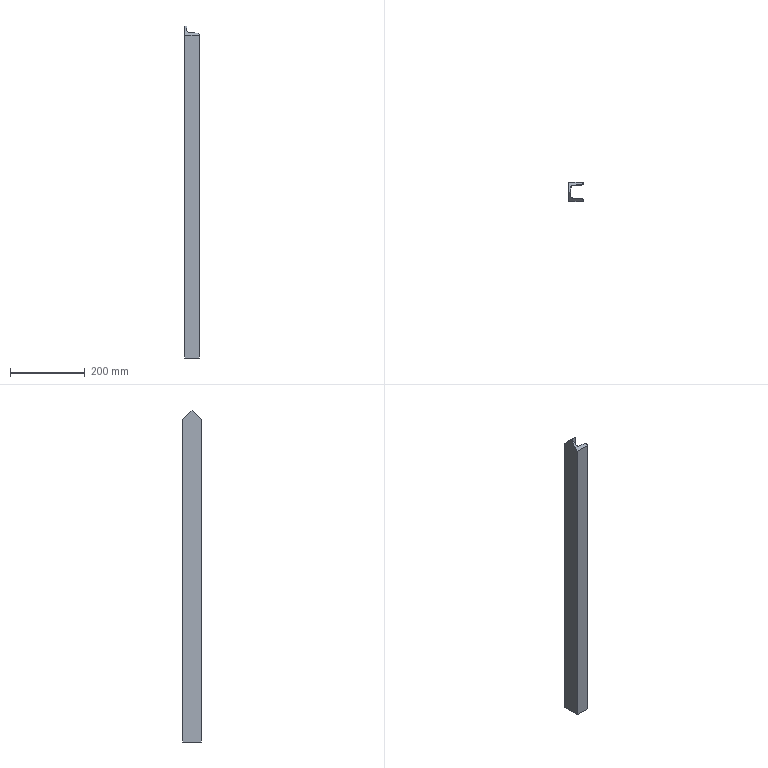Part | STEP file | DIN 1026-1 U 50 1785357045460 | 1 solid | 15 faces | box 38 x 50 x 885.962 mm | volume 617699 mm3 | plane 11 | cylinder 4 | commonest cylinder face diameters 7 x2 14 x2
STEP:
#1=CARTESIAN_POINT('',(0.,-0.000000005,935.962));
#2=VERTEX_POINT('',#1);
#3=CARTESIAN_POINT('',(5.,-0.000000005,935.962));
#4=VERTEX_POINT('',#3);
#5=CARTESIAN_POINT('',(9.5,-0.000000005,935.962));
#6=DIRECTION('',(1.,0.,0.));
#7=VECTOR('',#6,10.);
#8=LINE('',#5,#7);
#9=EDGE_CURVE('',#2,#4,#8,.T.);
#10=ORIENTED_EDGE('',*,*,#9,.T.);
#11=CARTESIAN_POINT('',(5.,10.418,925.544));
#12=VERTEX_POINT('',#11);
#13=CARTESIAN_POINT('',(5.,467.981,467.981));
#14=DIRECTION('',(0.,-0.7071,0.7071));
#15=VECTOR('',#14,10.);
#16=LINE('',#13,#15);
#17=EDGE_CURVE('',#12,#4,#16,.T.);
#18=ORIENTED_EDGE('',*,*,#17,.F.);
#19=CARTESIAN_POINT('',(11.442,17.395,918.566));
#20=VERTEX_POINT('',#19);
#21=CARTESIAN_POINT('',(12.,10.418,925.544));
#22=DIRECTION('',(0.,0.7071,0.7071));
#23=DIRECTION('',(0.,0.7071,-0.7071));
#24=AXIS2_PLACEMENT_3D('',#21,#22,#23);
#25=ELLIPSE('',#24,9.899,7.);
#26=EDGE_CURVE('',#20,#12,#25,.T.);
#27=ORIENTED_EDGE('',*,*,#26,.F.);
#28=CARTESIAN_POINT('',(34.779,19.262,916.699));
#29=VERTEX_POINT('',#28);
#30=CARTESIAN_POINT('',(89.258,23.621,912.341));
#31=DIRECTION('',(-0.9937,-0.07949,0.07949));
#32=VECTOR('',#31,10.);
#33=LINE('',#30,#32);
#34=EDGE_CURVE('',#29,#20,#33,.T.);
#35=ORIENTED_EDGE('',*,*,#34,.F.);
#36=CARTESIAN_POINT('',(38.,22.751,913.21));
#37=VERTEX_POINT('',#36);
#38=CARTESIAN_POINT('',(34.5,22.751,913.21));
#39=DIRECTION('',(0.,-0.7071,-0.7071));
#40=DIRECTION('',(0.,0.7071,-0.7071));
#41=AXIS2_PLACEMENT_3D('',#38,#39,#40);
#42=ELLIPSE('',#41,4.95,3.5);
#43=EDGE_CURVE('',#37,#29,#42,.T.);
#44=ORIENTED_EDGE('',*,*,#43,.F.);
#45=CARTESIAN_POINT('',(38.,25.,910.962));
#46=VERTEX_POINT('',#45);
#47=CARTESIAN_POINT('',(38.,474.231,461.731));
#48=DIRECTION('',(0.,-0.7071,0.7071));
#49=VECTOR('',#48,10.);
#50=LINE('',#47,#49);
#51=EDGE_CURVE('',#46,#37,#50,.T.);
#52=ORIENTED_EDGE('',*,*,#51,.F.);
#53=CARTESIAN_POINT('',(0.,25.,910.962));
#54=VERTEX_POINT('',#53);
#55=CARTESIAN_POINT('',(0.,25.,910.962));
#56=DIRECTION('',(1.,0.,0.));
#57=VECTOR('',#56,10.);
#58=LINE('',#55,#57);
#59=EDGE_CURVE('',#54,#46,#58,.T.);
#60=ORIENTED_EDGE('',*,*,#59,.F.);
#61=CARTESIAN_POINT('',(0.,467.981,467.981));
#62=DIRECTION('',(0.,0.7071,-0.7071));
#63=VECTOR('',#62,10.);
#64=LINE('',#61,#63);
#65=EDGE_CURVE('',#2,#54,#64,.T.);
#66=ORIENTED_EDGE('',*,*,#65,.F.);
#67=EDGE_LOOP('',(#10,#18,#27,#35,#44,#52,#60,#66));
#68=FACE_OUTER_BOUND('',#67,.T.);
#69=CARTESIAN_POINT('',(0.,467.981,467.981));
#70=DIRECTION('',(0.,-0.7071,-0.7071));
#71=DIRECTION('',(-1.,0.,0.));
#72=AXIS2_PLACEMENT_3D('',#69,#70,#71);
#73=PLANE('',#72);
#74=ADVANCED_FACE('',(#68),#73,.F.);
#75=ORIENTED_EDGE('',*,*,#34,.T.);
#76=CARTESIAN_POINT('',(11.442,17.395,50.));
#77=VERTEX_POINT('',#76);
#78=CARTESIAN_POINT('',(11.442,17.395,0.));
#79=DIRECTION('',(0.,0.,1.));
#80=VECTOR('',#79,10.);
#81=LINE('',#78,#80);
#82=EDGE_CURVE('',#77,#20,#81,.T.);
#83=ORIENTED_EDGE('',*,*,#82,.F.);
#84=CARTESIAN_POINT('',(34.779,19.262,50.));
#85=VERTEX_POINT('',#84);
#86=CARTESIAN_POINT('',(26.174,18.574,50.));
#87=DIRECTION('',(-0.9968,-0.07975,0.));
#88=VECTOR('',#87,10.);
#89=LINE('',#86,#88);
#90=EDGE_CURVE('',#85,#77,#89,.T.);
#91=ORIENTED_EDGE('',*,*,#90,.F.);
#92=CARTESIAN_POINT('',(34.779,19.262,0.));
#93=DIRECTION('',(0.,0.,1.));
#94=VECTOR('',#93,10.);
#95=LINE('',#92,#94);
#96=EDGE_CURVE('',#85,#29,#95,.T.);
#97=ORIENTED_EDGE('',*,*,#96,.T.);
#98=EDGE_LOOP('',(#75,#83,#91,#97));
#99=FACE_OUTER_BOUND('',#98,.T.);
#100=CARTESIAN_POINT('',(34.779,19.262,0.));
#101=DIRECTION('',(0.07975,-0.9968,0.));
#102=DIRECTION('',(0.,0.,-1.));
#103=AXIS2_PLACEMENT_3D('',#100,#101,#102);
#104=PLANE('',#103);
#105=ADVANCED_FACE('',(#99),#104,.T.);
#106=ORIENTED_EDGE('',*,*,#26,.T.);
#107=CARTESIAN_POINT('',(5.,10.418,50.));
#108=VERTEX_POINT('',#107);
#109=CARTESIAN_POINT('',(5.,10.418,0.));
#110=DIRECTION('',(0.,0.,1.));
#111=VECTOR('',#110,10.);
#112=LINE('',#109,#111);
#113=EDGE_CURVE('',#108,#12,#112,.T.);
#114=ORIENTED_EDGE('',*,*,#113,.F.);
#115=CARTESIAN_POINT('',(12.,10.418,50.));
#116=DIRECTION('',(0.,0.,1.));
#117=DIRECTION('',(-0.07975,0.9968,0.));
#118=AXIS2_PLACEMENT_3D('',#115,#116,#117);
#119=CIRCLE('',#118,7.);
#120=EDGE_CURVE('',#77,#108,#119,.T.);
#121=ORIENTED_EDGE('',*,*,#120,.F.);
#122=ORIENTED_EDGE('',*,*,#82,.T.);
#123=EDGE_LOOP('',(#106,#114,#121,#122));
#124=FACE_OUTER_BOUND('',#123,.T.);
#125=CARTESIAN_POINT('',(12.,10.418,0.));
#126=DIRECTION('',(0.,0.,1.));
#127=DIRECTION('',(-0.07975,0.9968,0.));
#128=AXIS2_PLACEMENT_3D('',#125,#126,#127);
#129=CYLINDRICAL_SURFACE('',#128,7.);
#130=ADVANCED_FACE('',(#124),#129,.F.);
#131=ORIENTED_EDGE('',*,*,#17,.T.);
#132=CARTESIAN_POINT('',(5.,-10.418,925.544));
#133=VERTEX_POINT('',#132);
#134=CARTESIAN_POINT('',(5.,-467.981,467.981));
#135=DIRECTION('',(0.,-0.7071,-0.7071));
#136=VECTOR('',#135,10.);
#137=LINE('',#134,#136);
#138=EDGE_CURVE('',#4,#133,#137,.T.);
#139=ORIENTED_EDGE('',*,*,#138,.T.);
#140=CARTESIAN_POINT('',(5.,-10.418,50.));
#141=VERTEX_POINT('',#140);
#142=CARTESIAN_POINT('',(5.,-10.418,0.));
#143=DIRECTION('',(0.,0.,1.));
#144=VECTOR('',#143,10.);
#145=LINE('',#142,#144);
#146=EDGE_CURVE('',#141,#133,#145,.T.);
#147=ORIENTED_EDGE('',*,*,#146,.F.);
#148=CARTESIAN_POINT('',(5.,0.,50.));
#149=DIRECTION('',(0.,-1.,0.));
#150=VECTOR('',#149,10.);
#151=LINE('',#148,#150);
#152=EDGE_CURVE('',#108,#141,#151,.T.);
#153=ORIENTED_EDGE('',*,*,#152,.F.);
#154=ORIENTED_EDGE('',*,*,#113,.T.);
#155=EDGE_LOOP('',(#131,#139,#147,#153,#154));
#156=FACE_OUTER_BOUND('',#155,.T.);
#157=CARTESIAN_POINT('',(5.,0.,0.));
#158=DIRECTION('',(1.,0.,0.));
#159=DIRECTION('',(0.,0.,-1.));
#160=AXIS2_PLACEMENT_3D('',#157,#158,#159);
#161=PLANE('',#160);
#162=ADVANCED_FACE('',(#156),#161,.T.);
#163=CARTESIAN_POINT('',(11.442,-17.395,918.566));
#164=VERTEX_POINT('',#163);
#165=CARTESIAN_POINT('',(12.,-10.418,925.544));
#166=DIRECTION('',(0.,-0.7071,0.7071));
#167=DIRECTION('',(0.,-0.7071,-0.7071));
#168=AXIS2_PLACEMENT_3D('',#165,#166,#167);
#169=ELLIPSE('',#168,9.899,7.);
#170=EDGE_CURVE('',#133,#164,#169,.T.);
#171=ORIENTED_EDGE('',*,*,#170,.F.);
#172=ORIENTED_EDGE('',*,*,#138,.F.);
#173=ORIENTED_EDGE('',*,*,#9,.F.);
#174=CARTESIAN_POINT('',(0.,-25.,910.962));
#175=VERTEX_POINT('',#174);
#176=CARTESIAN_POINT('',(0.,-467.981,467.981));
#177=DIRECTION('',(0.,0.7071,0.7071));
#178=VECTOR('',#177,10.);
#179=LINE('',#176,#178);
#180=EDGE_CURVE('',#175,#2,#179,.T.);
#181=ORIENTED_EDGE('',*,*,#180,.F.);
#182=CARTESIAN_POINT('',(38.,-25.,910.962));
#183=VERTEX_POINT('',#182);
#184=CARTESIAN_POINT('',(19.,-25.,910.962));
#185=DIRECTION('',(-1.,0.,0.));
#186=VECTOR('',#185,10.);
#187=LINE('',#184,#186);
#188=EDGE_CURVE('',#183,#175,#187,.T.);
#189=ORIENTED_EDGE('',*,*,#188,.F.);
#190=CARTESIAN_POINT('',(38.,-22.751,913.21));
#191=VERTEX_POINT('',#190);
#192=CARTESIAN_POINT('',(38.,-473.669,462.293));
#193=DIRECTION('',(0.,-0.7071,-0.7071));
#194=VECTOR('',#193,10.);
#195=LINE('',#192,#194);
#196=EDGE_CURVE('',#191,#183,#195,.T.);
#197=ORIENTED_EDGE('',*,*,#196,.F.);
#198=CARTESIAN_POINT('',(34.779,-19.262,916.699));
#199=VERTEX_POINT('',#198);
#200=CARTESIAN_POINT('',(34.5,-22.751,913.21));
#201=DIRECTION('',(0.,0.7071,-0.7071));
#202=DIRECTION('',(0.,-0.7071,-0.7071));
#203=AXIS2_PLACEMENT_3D('',#200,#201,#202);
#204=ELLIPSE('',#203,4.95,3.5);
#205=EDGE_CURVE('',#199,#191,#204,.T.);
#206=ORIENTED_EDGE('',*,*,#205,.F.);
#207=CARTESIAN_POINT('',(77.663,-22.693,913.269));
#208=DIRECTION('',(0.9937,-0.07949,-0.07949));
#209=VECTOR('',#208,10.);
#210=LINE('',#207,#209);
#211=EDGE_CURVE('',#164,#199,#210,.T.);
#212=ORIENTED_EDGE('',*,*,#211,.F.);
#213=EDGE_LOOP('',(#171,#172,#173,#181,#189,#197,#206,#212));
#214=FACE_OUTER_BOUND('',#213,.T.);
#215=CARTESIAN_POINT('',(0.,-467.981,467.981));
#216=DIRECTION('',(0.,0.7071,-0.7071));
#217=DIRECTION('',(-1.,0.,0.));
#218=AXIS2_PLACEMENT_3D('',#215,#216,#217);
#219=PLANE('',#218);
#220=ADVANCED_FACE('',(#214),#219,.F.);
#221=ORIENTED_EDGE('',*,*,#188,.T.);
#222=CARTESIAN_POINT('',(0.,-25.,50.));
#223=VERTEX_POINT('',#222);
#224=CARTESIAN_POINT('',(0.,-25.,0.));
#225=DIRECTION('',(0.,0.,1.));
#226=VECTOR('',#225,10.);
#227=LINE('',#224,#226);
#228=EDGE_CURVE('',#223,#175,#227,.T.);
#229=ORIENTED_EDGE('',*,*,#228,.F.);
#230=CARTESIAN_POINT('',(38.,-25.,50.));
#231=VERTEX_POINT('',#230);
#232=CARTESIAN_POINT('',(28.5,-25.,50.));
#233=DIRECTION('',(-1.,0.,0.));
#234=VECTOR('',#233,10.);
#235=LINE('',#232,#234);
#236=EDGE_CURVE('',#231,#223,#235,.T.);
#237=ORIENTED_EDGE('',*,*,#236,.F.);
#238=CARTESIAN_POINT('',(38.,-25.,0.));
#239=DIRECTION('',(0.,0.,1.));
#240=VECTOR('',#239,10.);
#241=LINE('',#238,#240);
#242=EDGE_CURVE('',#231,#183,#241,.T.);
#243=ORIENTED_EDGE('',*,*,#242,.T.);
#244=EDGE_LOOP('',(#221,#229,#237,#243));
#245=FACE_OUTER_BOUND('',#244,.T.);
#246=CARTESIAN_POINT('',(38.,-25.,0.));
#247=DIRECTION('',(0.,-1.,0.));
#248=DIRECTION('',(0.,0.,-1.));
#249=AXIS2_PLACEMENT_3D('',#246,#247,#248);
#250=PLANE('',#249);
#251=ADVANCED_FACE('',(#245),#250,.T.);
#252=ORIENTED_EDGE('',*,*,#65,.T.);
#253=CARTESIAN_POINT('',(0.,25.,50.));
#254=VERTEX_POINT('',#253);
#255=CARTESIAN_POINT('',(0.,25.,0.));
#256=DIRECTION('',(0.,0.,1.));
#257=VECTOR('',#256,10.);
#258=LINE('',#255,#257);
#259=EDGE_CURVE('',#254,#54,#258,.T.);
#260=ORIENTED_EDGE('',*,*,#259,.F.);
#261=CARTESIAN_POINT('',(0.,0.,50.));
#262=DIRECTION('',(0.,1.,0.));
#263=VECTOR('',#262,10.);
#264=LINE('',#261,#263);
#265=EDGE_CURVE('',#223,#254,#264,.T.);
#266=ORIENTED_EDGE('',*,*,#265,.F.);
#267=ORIENTED_EDGE('',*,*,#228,.T.);
#268=ORIENTED_EDGE('',*,*,#180,.T.);
#269=EDGE_LOOP('',(#252,#260,#266,#267,#268));
#270=FACE_OUTER_BOUND('',#269,.T.);
#271=CARTESIAN_POINT('',(0.,0.,0.));
#272=DIRECTION('',(-1.,0.,0.));
#273=DIRECTION('',(0.,0.,1.));
#274=AXIS2_PLACEMENT_3D('',#271,#272,#273);
#275=PLANE('',#274);
#276=ADVANCED_FACE('',(#270),#275,.T.);
#277=ORIENTED_EDGE('',*,*,#170,.T.);
#278=CARTESIAN_POINT('',(11.442,-17.395,50.));
#279=VERTEX_POINT('',#278);
#280=CARTESIAN_POINT('',(11.442,-17.395,0.));
#281=DIRECTION('',(0.,0.,1.));
#282=VECTOR('',#281,10.);
#283=LINE('',#280,#282);
#284=EDGE_CURVE('',#279,#164,#283,.T.);
#285=ORIENTED_EDGE('',*,*,#284,.F.);
#286=CARTESIAN_POINT('',(12.,-10.418,50.));
#287=DIRECTION('',(0.,0.,1.));
#288=DIRECTION('',(-1.,0.,0.));
#289=AXIS2_PLACEMENT_3D('',#286,#287,#288);
#290=CIRCLE('',#289,7.);
#291=EDGE_CURVE('',#141,#279,#290,.T.);
#292=ORIENTED_EDGE('',*,*,#291,.F.);
#293=ORIENTED_EDGE('',*,*,#146,.T.);
#294=EDGE_LOOP('',(#277,#285,#292,#293));
#295=FACE_OUTER_BOUND('',#294,.T.);
#296=CARTESIAN_POINT('',(12.,-10.418,0.));
#297=DIRECTION('',(0.,0.,1.));
#298=DIRECTION('',(-1.,0.,0.));
#299=AXIS2_PLACEMENT_3D('',#296,#297,#298);
#300=CYLINDRICAL_SURFACE('',#299,7.);
#301=ADVANCED_FACE('',(#295),#300,.F.);
#302=ORIENTED_EDGE('',*,*,#211,.T.);
#303=CARTESIAN_POINT('',(34.779,-19.262,50.));
#304=VERTEX_POINT('',#303);
#305=CARTESIAN_POINT('',(34.779,-19.262,0.));
#306=DIRECTION('',(0.,0.,1.));
#307=VECTOR('',#306,10.);
#308=LINE('',#305,#307);
#309=EDGE_CURVE('',#304,#199,#308,.T.);
#310=ORIENTED_EDGE('',*,*,#309,.F.);
#311=CARTESIAN_POINT('',(14.505,-17.64,50.));
#312=DIRECTION('',(0.9968,-0.07975,0.));
#313=VECTOR('',#312,10.);
#314=LINE('',#311,#313);
#315=EDGE_CURVE('',#279,#304,#314,.T.);
#316=ORIENTED_EDGE('',*,*,#315,.F.);
#317=ORIENTED_EDGE('',*,*,#284,.T.);
#318=EDGE_LOOP('',(#302,#310,#316,#317));
#319=FACE_OUTER_BOUND('',#318,.T.);
#320=CARTESIAN_POINT('',(11.442,-17.395,0.));
#321=DIRECTION('',(0.07975,0.9968,0.));
#322=DIRECTION('',(0.,0.,1.));
#323=AXIS2_PLACEMENT_3D('',#320,#321,#322);
#324=PLANE('',#323);
#325=ADVANCED_FACE('',(#319),#324,.T.);
#326=ORIENTED_EDGE('',*,*,#205,.T.);
#327=CARTESIAN_POINT('',(38.,-22.751,50.));
#328=VERTEX_POINT('',#327);
#329=CARTESIAN_POINT('',(38.,-22.751,0.));
#330=DIRECTION('',(0.,0.,1.));
#331=VECTOR('',#330,10.);
#332=LINE('',#329,#331);
#333=EDGE_CURVE('',#328,#191,#332,.T.);
#334=ORIENTED_EDGE('',*,*,#333,.F.);
#335=CARTESIAN_POINT('',(34.5,-22.751,50.));
#336=DIRECTION('',(0.,0.,-1.));
#337=DIRECTION('',(-1.,0.,0.));
#338=AXIS2_PLACEMENT_3D('',#335,#336,#337);
#339=CIRCLE('',#338,3.5);
#340=EDGE_CURVE('',#304,#328,#339,.T.);
#341=ORIENTED_EDGE('',*,*,#340,.F.);
#342=ORIENTED_EDGE('',*,*,#309,.T.);
#343=EDGE_LOOP('',(#326,#334,#341,#342));
#344=FACE_OUTER_BOUND('',#343,.T.);
#345=CARTESIAN_POINT('',(34.5,-22.751,0.));
#346=DIRECTION('',(0.,0.,1.));
#347=DIRECTION('',(-1.,0.,0.));
#348=AXIS2_PLACEMENT_3D('',#345,#346,#347);
#349=CYLINDRICAL_SURFACE('',#348,3.5);
#350=ADVANCED_FACE('',(#344),#349,.T.);
#351=ORIENTED_EDGE('',*,*,#196,.T.);
#352=ORIENTED_EDGE('',*,*,#242,.F.);
#353=CARTESIAN_POINT('',(38.,-11.376,50.));
#354=DIRECTION('',(0.,-1.,0.));
#355=VECTOR('',#354,10.);
#356=LINE('',#353,#355);
#357=EDGE_CURVE('',#328,#231,#356,.T.);
#358=ORIENTED_EDGE('',*,*,#357,.F.);
#359=ORIENTED_EDGE('',*,*,#333,.T.);
#360=EDGE_LOOP('',(#351,#352,#358,#359));
#361=FACE_OUTER_BOUND('',#360,.T.);
#362=CARTESIAN_POINT('',(38.,-22.751,0.));
#363=DIRECTION('',(1.,0.,0.));
#364=DIRECTION('',(0.,0.,-1.));
#365=AXIS2_PLACEMENT_3D('',#362,#363,#364);
#366=PLANE('',#365);
#367=ADVANCED_FACE('',(#361),#366,.T.);
#368=ORIENTED_EDGE('',*,*,#59,.T.);
#369=CARTESIAN_POINT('',(38.,25.,50.));
#370=VERTEX_POINT('',#369);
#371=CARTESIAN_POINT('',(38.,25.,0.));
#372=DIRECTION('',(0.,0.,1.));
#373=VECTOR('',#372,10.);
#374=LINE('',#371,#373);
#375=EDGE_CURVE('',#370,#46,#374,.T.);
#376=ORIENTED_EDGE('',*,*,#375,.F.);
#377=CARTESIAN_POINT('',(9.5,25.,50.));
#378=DIRECTION('',(1.,0.,0.));
#379=VECTOR('',#378,10.);
#380=LINE('',#377,#379);
#381=EDGE_CURVE('',#254,#370,#380,.T.);
#382=ORIENTED_EDGE('',*,*,#381,.F.);
#383=ORIENTED_EDGE('',*,*,#259,.T.);
#384=EDGE_LOOP('',(#368,#376,#382,#383));
#385=FACE_OUTER_BOUND('',#384,.T.);
#386=CARTESIAN_POINT('',(0.,25.,0.));
#387=DIRECTION('',(0.,1.,0.));
#388=DIRECTION('',(0.,0.,1.));
#389=AXIS2_PLACEMENT_3D('',#386,#387,#388);
#390=PLANE('',#389);
#391=ADVANCED_FACE('',(#385),#390,.T.);
#392=ORIENTED_EDGE('',*,*,#51,.T.);
#393=CARTESIAN_POINT('',(38.,22.751,50.));
#394=VERTEX_POINT('',#393);
#395=CARTESIAN_POINT('',(38.,22.751,0.));
#396=DIRECTION('',(0.,0.,1.));
#397=VECTOR('',#396,10.);
#398=LINE('',#395,#397);
#399=EDGE_CURVE('',#394,#37,#398,.T.);
#400=ORIENTED_EDGE('',*,*,#399,.F.);
#401=CARTESIAN_POINT('',(38.,12.5,50.));
#402=DIRECTION('',(0.,-1.,0.));
#403=VECTOR('',#402,10.);
#404=LINE('',#401,#403);
#405=EDGE_CURVE('',#370,#394,#404,.T.);
#406=ORIENTED_EDGE('',*,*,#405,.F.);
#407=ORIENTED_EDGE('',*,*,#375,.T.);
#408=EDGE_LOOP('',(#392,#400,#406,#407));
#409=FACE_OUTER_BOUND('',#408,.T.);
#410=CARTESIAN_POINT('',(38.,25.,0.));
#411=DIRECTION('',(1.,0.,0.));
#412=DIRECTION('',(0.,0.,-1.));
#413=AXIS2_PLACEMENT_3D('',#410,#411,#412);
#414=PLANE('',#413);
#415=ADVANCED_FACE('',(#409),#414,.T.);
#416=ORIENTED_EDGE('',*,*,#43,.T.);
#417=ORIENTED_EDGE('',*,*,#96,.F.);
#418=CARTESIAN_POINT('',(34.5,22.751,50.));
#419=DIRECTION('',(0.,0.,-1.));
#420=DIRECTION('',(-0.07975,0.9968,0.));
#421=AXIS2_PLACEMENT_3D('',#418,#419,#420);
#422=CIRCLE('',#421,3.5);
#423=EDGE_CURVE('',#394,#85,#422,.T.);
#424=ORIENTED_EDGE('',*,*,#423,.F.);
#425=ORIENTED_EDGE('',*,*,#399,.T.);
#426=EDGE_LOOP('',(#416,#417,#424,#425));
#427=FACE_OUTER_BOUND('',#426,.T.);
#428=CARTESIAN_POINT('',(34.5,22.751,0.));
#429=DIRECTION('',(0.,0.,1.));
#430=DIRECTION('',(-0.07975,0.9968,0.));
#431=AXIS2_PLACEMENT_3D('',#428,#429,#430);
#432=CYLINDRICAL_SURFACE('',#431,3.5);
#433=ADVANCED_FACE('',(#427),#432,.T.);
#434=ORIENTED_EDGE('',*,*,#381,.T.);
#435=ORIENTED_EDGE('',*,*,#405,.T.);
#436=ORIENTED_EDGE('',*,*,#423,.T.);
#437=ORIENTED_EDGE('',*,*,#90,.T.);
#438=ORIENTED_EDGE('',*,*,#120,.T.);
#439=ORIENTED_EDGE('',*,*,#152,.T.);
#440=ORIENTED_EDGE('',*,*,#291,.T.);
#441=ORIENTED_EDGE('',*,*,#315,.T.);
#442=ORIENTED_EDGE('',*,*,#340,.T.);
#443=ORIENTED_EDGE('',*,*,#357,.T.);
#444=ORIENTED_EDGE('',*,*,#236,.T.);
#445=ORIENTED_EDGE('',*,*,#265,.T.);
#446=EDGE_LOOP('',(#434,#435,#436,#437,#438,#439,#440,#441,#442,#443,#444,#445));
#447=FACE_OUTER_BOUND('',#446,.T.);
#448=CARTESIAN_POINT('',(19.,0.,50.));
#449=DIRECTION('',(0.,0.,1.));
#450=DIRECTION('',(1.,0.,0.));
#451=AXIS2_PLACEMENT_3D('',#448,#449,#450);
#452=PLANE('',#451);
#453=ADVANCED_FACE('',(#447),#452,.F.);
#454=CLOSED_SHELL('',(#74,#105,#130,#162,#220,#251,#276,#301,#325,#350,#367,#391,#415,#433,#453));
#455=MANIFOLD_SOLID_BREP('',#454);
#456=(LENGTH_UNIT()NAMED_UNIT(*)SI_UNIT(.MILLI.,.METRE.));
#457=UNCERTAINTY_MEASURE_WITH_UNIT(LENGTH_MEASURE(0.01),#456,'','');
#458=(NAMED_UNIT(*)PLANE_ANGLE_UNIT()SI_UNIT($,.RADIAN.));
#459=(NAMED_UNIT(*)SI_UNIT($,.STERADIAN.)SOLID_ANGLE_UNIT());
#460=(GEOMETRIC_REPRESENTATION_CONTEXT(3)GLOBAL_UNCERTAINTY_ASSIGNED_CONTEXT((#457))GLOBAL_UNIT_ASSIGNED_CONTEXT((#456,#458,#459))REPRESENTATION_CONTEXT('',''));
#461=ADVANCED_BREP_SHAPE_REPRESENTATION('',(#455),#460);